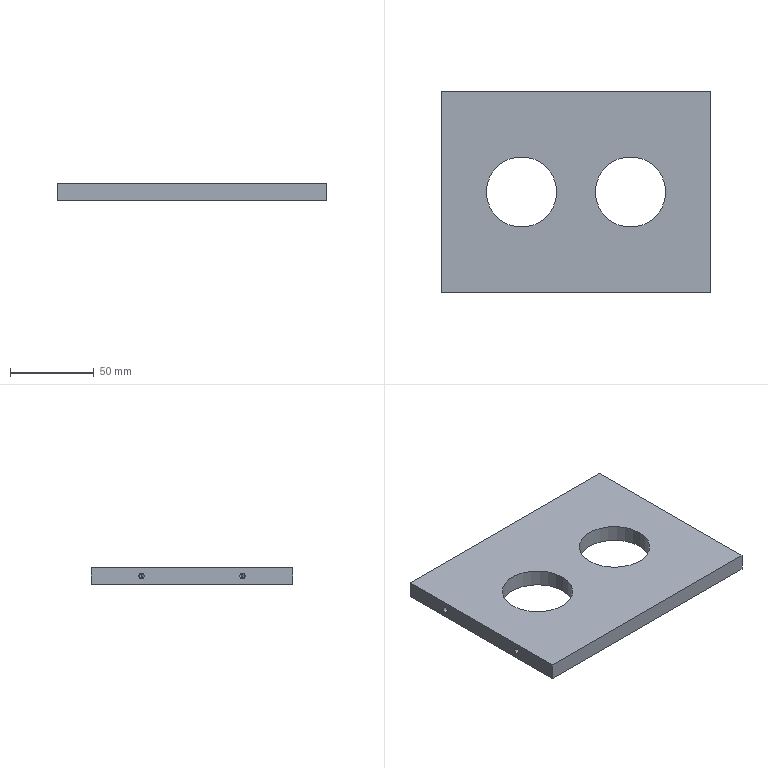Part | NX | 1 solid | 26 faces | box 160 x 120 x 10 mm | volume 163934 mm3 | cylinder 12 | cone 8 | plane 6 | commonest cylinder face diameters 3.3 x8 42 x4
STEP:
#1=CARTESIAN_POINT('',(-69.9,-30.,3.35));
#2=VERTEX_POINT('',#1);
#3=CARTESIAN_POINT('',(-69.9,-30.,6.65));
#4=VERTEX_POINT('',#3);
#5=CARTESIAN_POINT('',(-69.9,-30.,5.));
#6=DIRECTION('',(-1.,0.,0.));
#7=DIRECTION('',(0.,0.,1.));
#8=AXIS2_PLACEMENT_3D('',#5,#6,#7);
#9=CIRCLE('',#8,1.65);
#10=EDGE_CURVE('',#2,#4,#9,.T.);
#11=ORIENTED_EDGE('',*,*,#10,.F.);
#12=CARTESIAN_POINT('',(-80.,-30.,3.35));
#13=VERTEX_POINT('',#12);
#14=CARTESIAN_POINT('',(-80.,-30.,3.35));
#15=DIRECTION('',(-1.,0.,0.));
#16=VECTOR('',#15,1.);
#17=LINE('',#14,#16);
#18=EDGE_CURVE('',#2,#13,#17,.T.);
#19=ORIENTED_EDGE('',*,*,#18,.T.);
#20=CARTESIAN_POINT('',(-80.,-30.,6.65));
#21=VERTEX_POINT('',#20);
#22=CARTESIAN_POINT('',(-80.,-30.,5.));
#23=DIRECTION('',(-1.,0.,0.));
#24=DIRECTION('',(0.,0.,1.));
#25=AXIS2_PLACEMENT_3D('',#22,#23,#24);
#26=CIRCLE('',#25,1.65);
#27=EDGE_CURVE('',#13,#21,#26,.T.);
#28=ORIENTED_EDGE('',*,*,#27,.T.);
#29=CARTESIAN_POINT('',(-80.,-30.,6.65));
#30=DIRECTION('',(-1.,0.,0.));
#31=VECTOR('',#30,1.);
#32=LINE('',#29,#31);
#33=EDGE_CURVE('',#4,#21,#32,.T.);
#34=ORIENTED_EDGE('',*,*,#33,.F.);
#35=EDGE_LOOP('',(#11,#19,#28,#34));
#36=FACE_OUTER_BOUND('',#35,.T.);
#37=CARTESIAN_POINT('',(-80.,-30.,5.));
#38=DIRECTION('',(-1.,0.,0.));
#39=DIRECTION('',(0.,0.,1.));
#40=AXIS2_PLACEMENT_3D('',#37,#38,#39);
#41=CYLINDRICAL_SURFACE('',#40,1.65);
#42=ADVANCED_FACE('',(#36),#41,.F.);
#43=CARTESIAN_POINT('',(-68.909,-30.,5.));
#44=VERTEX_POINT('',#43);
#45=CARTESIAN_POINT('',(-69.9,-30.,6.65));
#46=DIRECTION('',(-0.515,0.,0.8572));
#47=VECTOR('',#46,1.);
#48=LINE('',#45,#47);
#49=EDGE_CURVE('',#44,#4,#48,.T.);
#50=ORIENTED_EDGE('',*,*,#49,.F.);
#51=CARTESIAN_POINT('',(-69.9,-30.,3.35));
#52=DIRECTION('',(-0.515,0.,-0.8572));
#53=VECTOR('',#52,1.);
#54=LINE('',#51,#53);
#55=EDGE_CURVE('',#44,#2,#54,.T.);
#56=ORIENTED_EDGE('',*,*,#55,.T.);
#57=ORIENTED_EDGE('',*,*,#10,.T.);
#58=EDGE_LOOP('',(#50,#56,#57));
#59=FACE_OUTER_BOUND('',#58,.T.);
#60=CARTESIAN_POINT('',(-69.9,-30.,5.));
#61=DIRECTION('',(-1.,0.,0.));
#62=DIRECTION('',(0.,0.,1.));
#63=AXIS2_PLACEMENT_3D('',#60,#61,#62);
#64=CONICAL_SURFACE('',#63,1.65,59.);
#65=ADVANCED_FACE('',(#59),#64,.F.);
#66=CARTESIAN_POINT('',(-69.9,30.,3.35));
#67=VERTEX_POINT('',#66);
#68=CARTESIAN_POINT('',(-69.9,30.,6.65));
#69=VERTEX_POINT('',#68);
#70=CARTESIAN_POINT('',(-69.9,30.,5.));
#71=DIRECTION('',(-1.,0.,0.));
#72=DIRECTION('',(0.,0.,1.));
#73=AXIS2_PLACEMENT_3D('',#70,#71,#72);
#74=CIRCLE('',#73,1.65);
#75=EDGE_CURVE('',#67,#69,#74,.T.);
#76=ORIENTED_EDGE('',*,*,#75,.F.);
#77=CARTESIAN_POINT('',(-80.,30.,3.35));
#78=VERTEX_POINT('',#77);
#79=CARTESIAN_POINT('',(-80.,30.,3.35));
#80=DIRECTION('',(-1.,0.,0.));
#81=VECTOR('',#80,1.);
#82=LINE('',#79,#81);
#83=EDGE_CURVE('',#67,#78,#82,.T.);
#84=ORIENTED_EDGE('',*,*,#83,.T.);
#85=CARTESIAN_POINT('',(-80.,30.,6.65));
#86=VERTEX_POINT('',#85);
#87=CARTESIAN_POINT('',(-80.,30.,5.));
#88=DIRECTION('',(-1.,0.,0.));
#89=DIRECTION('',(0.,0.,1.));
#90=AXIS2_PLACEMENT_3D('',#87,#88,#89);
#91=CIRCLE('',#90,1.65);
#92=EDGE_CURVE('',#78,#86,#91,.T.);
#93=ORIENTED_EDGE('',*,*,#92,.T.);
#94=CARTESIAN_POINT('',(-80.,30.,6.65));
#95=DIRECTION('',(-1.,0.,0.));
#96=VECTOR('',#95,1.);
#97=LINE('',#94,#96);
#98=EDGE_CURVE('',#69,#86,#97,.T.);
#99=ORIENTED_EDGE('',*,*,#98,.F.);
#100=EDGE_LOOP('',(#76,#84,#93,#99));
#101=FACE_OUTER_BOUND('',#100,.T.);
#102=CARTESIAN_POINT('',(-80.,30.,5.));
#103=DIRECTION('',(-1.,0.,0.));
#104=DIRECTION('',(0.,0.,1.));
#105=AXIS2_PLACEMENT_3D('',#102,#103,#104);
#106=CYLINDRICAL_SURFACE('',#105,1.65);
#107=ADVANCED_FACE('',(#101),#106,.F.);
#108=CARTESIAN_POINT('',(-68.909,30.,5.));
#109=VERTEX_POINT('',#108);
#110=CARTESIAN_POINT('',(-69.9,30.,6.65));
#111=DIRECTION('',(-0.515,0.,0.8572));
#112=VECTOR('',#111,1.);
#113=LINE('',#110,#112);
#114=EDGE_CURVE('',#109,#69,#113,.T.);
#115=ORIENTED_EDGE('',*,*,#114,.F.);
#116=CARTESIAN_POINT('',(-69.9,30.,3.35));
#117=DIRECTION('',(-0.515,0.,-0.8572));
#118=VECTOR('',#117,1.);
#119=LINE('',#116,#118);
#120=EDGE_CURVE('',#109,#67,#119,.T.);
#121=ORIENTED_EDGE('',*,*,#120,.T.);
#122=ORIENTED_EDGE('',*,*,#75,.T.);
#123=EDGE_LOOP('',(#115,#121,#122));
#124=FACE_OUTER_BOUND('',#123,.T.);
#125=CARTESIAN_POINT('',(-69.9,30.,5.));
#126=DIRECTION('',(-1.,0.,0.));
#127=DIRECTION('',(0.,0.,1.));
#128=AXIS2_PLACEMENT_3D('',#125,#126,#127);
#129=CONICAL_SURFACE('',#128,1.65,59.);
#130=ADVANCED_FACE('',(#124),#129,.F.);
#131=CARTESIAN_POINT('',(69.9,-30.,6.65));
#132=VERTEX_POINT('',#131);
#133=CARTESIAN_POINT('',(69.9,-30.,3.35));
#134=VERTEX_POINT('',#133);
#135=CARTESIAN_POINT('',(69.9,-30.,5.));
#136=DIRECTION('',(1.,0.,0.));
#137=DIRECTION('',(0.,0.,-1.));
#138=AXIS2_PLACEMENT_3D('',#135,#136,#137);
#139=CIRCLE('',#138,1.65);
#140=EDGE_CURVE('',#132,#134,#139,.T.);
#141=ORIENTED_EDGE('',*,*,#140,.F.);
#142=CARTESIAN_POINT('',(80.,-30.,6.65));
#143=VERTEX_POINT('',#142);
#144=CARTESIAN_POINT('',(80.,-30.,6.65));
#145=DIRECTION('',(-1.,0.,0.));
#146=VECTOR('',#145,1.);
#147=LINE('',#144,#146);
#148=EDGE_CURVE('',#143,#132,#147,.T.);
#149=ORIENTED_EDGE('',*,*,#148,.F.);
#150=CARTESIAN_POINT('',(80.,-30.,3.35));
#151=VERTEX_POINT('',#150);
#152=CARTESIAN_POINT('',(80.,-30.,5.));
#153=DIRECTION('',(1.,0.,0.));
#154=DIRECTION('',(0.,0.,-1.));
#155=AXIS2_PLACEMENT_3D('',#152,#153,#154);
#156=CIRCLE('',#155,1.65);
#157=EDGE_CURVE('',#143,#151,#156,.T.);
#158=ORIENTED_EDGE('',*,*,#157,.T.);
#159=CARTESIAN_POINT('',(80.,-30.,3.35));
#160=DIRECTION('',(-1.,0.,0.));
#161=VECTOR('',#160,1.);
#162=LINE('',#159,#161);
#163=EDGE_CURVE('',#151,#134,#162,.T.);
#164=ORIENTED_EDGE('',*,*,#163,.T.);
#165=EDGE_LOOP('',(#141,#149,#158,#164));
#166=FACE_OUTER_BOUND('',#165,.T.);
#167=CARTESIAN_POINT('',(80.,-30.,5.));
#168=DIRECTION('',(1.,0.,0.));
#169=DIRECTION('',(0.,0.,-1.));
#170=AXIS2_PLACEMENT_3D('',#167,#168,#169);
#171=CYLINDRICAL_SURFACE('',#170,1.65);
#172=ADVANCED_FACE('',(#166),#171,.F.);
#173=CARTESIAN_POINT('',(68.909,-30.,5.));
#174=VERTEX_POINT('',#173);
#175=CARTESIAN_POINT('',(69.9,-30.,3.35));
#176=DIRECTION('',(-0.515,0.,0.8572));
#177=VECTOR('',#176,1.);
#178=LINE('',#175,#177);
#179=EDGE_CURVE('',#134,#174,#178,.T.);
#180=ORIENTED_EDGE('',*,*,#179,.T.);
#181=CARTESIAN_POINT('',(69.9,-30.,6.65));
#182=DIRECTION('',(-0.515,0.,-0.8572));
#183=VECTOR('',#182,1.);
#184=LINE('',#181,#183);
#185=EDGE_CURVE('',#132,#174,#184,.T.);
#186=ORIENTED_EDGE('',*,*,#185,.F.);
#187=ORIENTED_EDGE('',*,*,#140,.T.);
#188=EDGE_LOOP('',(#180,#186,#187));
#189=FACE_OUTER_BOUND('',#188,.T.);
#190=CARTESIAN_POINT('',(69.9,-30.,5.));
#191=DIRECTION('',(1.,0.,0.));
#192=DIRECTION('',(0.,0.,-1.));
#193=AXIS2_PLACEMENT_3D('',#190,#191,#192);
#194=CONICAL_SURFACE('',#193,1.65,59.);
#195=ADVANCED_FACE('',(#189),#194,.F.);
#196=CARTESIAN_POINT('',(69.9,30.,6.65));
#197=VERTEX_POINT('',#196);
#198=CARTESIAN_POINT('',(69.9,30.,3.35));
#199=VERTEX_POINT('',#198);
#200=CARTESIAN_POINT('',(69.9,30.,5.));
#201=DIRECTION('',(1.,0.,0.));
#202=DIRECTION('',(0.,0.,-1.));
#203=AXIS2_PLACEMENT_3D('',#200,#201,#202);
#204=CIRCLE('',#203,1.65);
#205=EDGE_CURVE('',#197,#199,#204,.T.);
#206=ORIENTED_EDGE('',*,*,#205,.F.);
#207=CARTESIAN_POINT('',(80.,30.,6.65));
#208=VERTEX_POINT('',#207);
#209=CARTESIAN_POINT('',(80.,30.,6.65));
#210=DIRECTION('',(-1.,0.,0.));
#211=VECTOR('',#210,1.);
#212=LINE('',#209,#211);
#213=EDGE_CURVE('',#208,#197,#212,.T.);
#214=ORIENTED_EDGE('',*,*,#213,.F.);
#215=CARTESIAN_POINT('',(80.,30.,3.35));
#216=VERTEX_POINT('',#215);
#217=CARTESIAN_POINT('',(80.,30.,5.));
#218=DIRECTION('',(1.,0.,0.));
#219=DIRECTION('',(0.,0.,-1.));
#220=AXIS2_PLACEMENT_3D('',#217,#218,#219);
#221=CIRCLE('',#220,1.65);
#222=EDGE_CURVE('',#208,#216,#221,.T.);
#223=ORIENTED_EDGE('',*,*,#222,.T.);
#224=CARTESIAN_POINT('',(80.,30.,3.35));
#225=DIRECTION('',(-1.,0.,0.));
#226=VECTOR('',#225,1.);
#227=LINE('',#224,#226);
#228=EDGE_CURVE('',#216,#199,#227,.T.);
#229=ORIENTED_EDGE('',*,*,#228,.T.);
#230=EDGE_LOOP('',(#206,#214,#223,#229));
#231=FACE_OUTER_BOUND('',#230,.T.);
#232=CARTESIAN_POINT('',(80.,30.,5.));
#233=DIRECTION('',(1.,0.,0.));
#234=DIRECTION('',(0.,0.,-1.));
#235=AXIS2_PLACEMENT_3D('',#232,#233,#234);
#236=CYLINDRICAL_SURFACE('',#235,1.65);
#237=ADVANCED_FACE('',(#231),#236,.F.);
#238=CARTESIAN_POINT('',(68.909,30.,5.));
#239=VERTEX_POINT('',#238);
#240=CARTESIAN_POINT('',(69.9,30.,3.35));
#241=DIRECTION('',(-0.515,0.,0.8572));
#242=VECTOR('',#241,1.);
#243=LINE('',#240,#242);
#244=EDGE_CURVE('',#199,#239,#243,.T.);
#245=ORIENTED_EDGE('',*,*,#244,.T.);
#246=CARTESIAN_POINT('',(69.9,30.,6.65));
#247=DIRECTION('',(-0.515,0.,-0.8572));
#248=VECTOR('',#247,1.);
#249=LINE('',#246,#248);
#250=EDGE_CURVE('',#197,#239,#249,.T.);
#251=ORIENTED_EDGE('',*,*,#250,.F.);
#252=ORIENTED_EDGE('',*,*,#205,.T.);
#253=EDGE_LOOP('',(#245,#251,#252));
#254=FACE_OUTER_BOUND('',#253,.T.);
#255=CARTESIAN_POINT('',(69.9,30.,5.));
#256=DIRECTION('',(1.,0.,0.));
#257=DIRECTION('',(0.,0.,-1.));
#258=AXIS2_PLACEMENT_3D('',#255,#256,#257);
#259=CONICAL_SURFACE('',#258,1.65,59.);
#260=ADVANCED_FACE('',(#254),#259,.F.);
#261=CARTESIAN_POINT('',(-53.5,0.,10.));
#262=VERTEX_POINT('',#261);
#263=CARTESIAN_POINT('',(-11.5,0.,10.));
#264=VERTEX_POINT('',#263);
#265=CARTESIAN_POINT('',(-32.5,0.,10.));
#266=DIRECTION('',(0.,0.,1.));
#267=DIRECTION('',(1.,0.,0.));
#268=AXIS2_PLACEMENT_3D('',#265,#266,#267);
#269=CIRCLE('',#268,21.);
#270=EDGE_CURVE('',#262,#264,#269,.T.);
#271=ORIENTED_EDGE('',*,*,#270,.T.);
#272=CARTESIAN_POINT('',(-11.5,0.,0.));
#273=VERTEX_POINT('',#272);
#274=CARTESIAN_POINT('',(-11.5,0.,10.));
#275=DIRECTION('',(0.,0.,1.));
#276=VECTOR('',#275,1.);
#277=LINE('',#274,#276);
#278=EDGE_CURVE('',#273,#264,#277,.T.);
#279=ORIENTED_EDGE('',*,*,#278,.F.);
#280=CARTESIAN_POINT('',(-53.5,0.,0.));
#281=VERTEX_POINT('',#280);
#282=CARTESIAN_POINT('',(-32.5,0.,0.));
#283=DIRECTION('',(0.,0.,1.));
#284=DIRECTION('',(1.,0.,0.));
#285=AXIS2_PLACEMENT_3D('',#282,#283,#284);
#286=CIRCLE('',#285,21.);
#287=EDGE_CURVE('',#281,#273,#286,.T.);
#288=ORIENTED_EDGE('',*,*,#287,.F.);
#289=CARTESIAN_POINT('',(-53.5,0.,10.));
#290=DIRECTION('',(0.,0.,1.));
#291=VECTOR('',#290,1.);
#292=LINE('',#289,#291);
#293=EDGE_CURVE('',#281,#262,#292,.T.);
#294=ORIENTED_EDGE('',*,*,#293,.T.);
#295=EDGE_LOOP('',(#271,#279,#288,#294));
#296=FACE_OUTER_BOUND('',#295,.T.);
#297=CARTESIAN_POINT('',(-32.5,0.,10.));
#298=DIRECTION('',(0.,0.,-1.));
#299=DIRECTION('',(-1.,0.,0.));
#300=AXIS2_PLACEMENT_3D('',#297,#298,#299);
#301=CYLINDRICAL_SURFACE('',#300,21.);
#302=ADVANCED_FACE('',(#296),#301,.F.);
#303=CARTESIAN_POINT('',(11.5,0.,10.));
#304=VERTEX_POINT('',#303);
#305=CARTESIAN_POINT('',(53.5,0.,10.));
#306=VERTEX_POINT('',#305);
#307=CARTESIAN_POINT('',(32.5,0.,10.));
#308=DIRECTION('',(0.,0.,1.));
#309=DIRECTION('',(1.,0.,0.));
#310=AXIS2_PLACEMENT_3D('',#307,#308,#309);
#311=CIRCLE('',#310,21.);
#312=EDGE_CURVE('',#304,#306,#311,.T.);
#313=ORIENTED_EDGE('',*,*,#312,.T.);
#314=CARTESIAN_POINT('',(53.5,0.,0.));
#315=VERTEX_POINT('',#314);
#316=CARTESIAN_POINT('',(53.5,0.,10.));
#317=DIRECTION('',(0.,0.,1.));
#318=VECTOR('',#317,1.);
#319=LINE('',#316,#318);
#320=EDGE_CURVE('',#315,#306,#319,.T.);
#321=ORIENTED_EDGE('',*,*,#320,.F.);
#322=CARTESIAN_POINT('',(11.5,0.,0.));
#323=VERTEX_POINT('',#322);
#324=CARTESIAN_POINT('',(32.5,0.,0.));
#325=DIRECTION('',(0.,0.,1.));
#326=DIRECTION('',(1.,0.,0.));
#327=AXIS2_PLACEMENT_3D('',#324,#325,#326);
#328=CIRCLE('',#327,21.);
#329=EDGE_CURVE('',#323,#315,#328,.T.);
#330=ORIENTED_EDGE('',*,*,#329,.F.);
#331=CARTESIAN_POINT('',(11.5,0.,10.));
#332=DIRECTION('',(0.,0.,1.));
#333=VECTOR('',#332,1.);
#334=LINE('',#331,#333);
#335=EDGE_CURVE('',#323,#304,#334,.T.);
#336=ORIENTED_EDGE('',*,*,#335,.T.);
#337=EDGE_LOOP('',(#313,#321,#330,#336));
#338=FACE_OUTER_BOUND('',#337,.T.);
#339=CARTESIAN_POINT('',(32.5,0.,10.));
#340=DIRECTION('',(0.,0.,-1.));
#341=DIRECTION('',(-1.,0.,0.));
#342=AXIS2_PLACEMENT_3D('',#339,#340,#341);
#343=CYLINDRICAL_SURFACE('',#342,21.);
#344=ADVANCED_FACE('',(#338),#343,.F.);
#345=ORIENTED_EDGE('',*,*,#312,.F.);
#346=CARTESIAN_POINT('',(32.5,0.,10.));
#347=DIRECTION('',(0.,0.,1.));
#348=DIRECTION('',(1.,0.,0.));
#349=AXIS2_PLACEMENT_3D('',#346,#347,#348);
#350=CIRCLE('',#349,21.);
#351=EDGE_CURVE('',#306,#304,#350,.T.);
#352=ORIENTED_EDGE('',*,*,#351,.F.);
#353=EDGE_LOOP('',(#345,#352));
#354=FACE_BOUND('',#353,.T.);
#355=CARTESIAN_POINT('',(80.,-60.,10.));
#356=VERTEX_POINT('',#355);
#357=CARTESIAN_POINT('',(80.,60.,10.));
#358=VERTEX_POINT('',#357);
#359=CARTESIAN_POINT('',(80.,60.,10.));
#360=DIRECTION('',(0.,1.,0.));
#361=VECTOR('',#360,1.);
#362=LINE('',#359,#361);
#363=EDGE_CURVE('',#356,#358,#362,.T.);
#364=ORIENTED_EDGE('',*,*,#363,.T.);
#365=CARTESIAN_POINT('',(-80.,60.,10.));
#366=VERTEX_POINT('',#365);
#367=CARTESIAN_POINT('',(-80.,60.,10.));
#368=DIRECTION('',(-1.,0.,0.));
#369=VECTOR('',#368,1.);
#370=LINE('',#367,#369);
#371=EDGE_CURVE('',#358,#366,#370,.T.);
#372=ORIENTED_EDGE('',*,*,#371,.T.);
#373=CARTESIAN_POINT('',(-80.,-60.,10.));
#374=VERTEX_POINT('',#373);
#375=CARTESIAN_POINT('',(-80.,60.,10.));
#376=DIRECTION('',(0.,-1.,0.));
#377=VECTOR('',#376,1.);
#378=LINE('',#375,#377);
#379=EDGE_CURVE('',#366,#374,#378,.T.);
#380=ORIENTED_EDGE('',*,*,#379,.T.);
#381=CARTESIAN_POINT('',(-80.,-60.,10.));
#382=DIRECTION('',(1.,0.,0.));
#383=VECTOR('',#382,1.);
#384=LINE('',#381,#383);
#385=EDGE_CURVE('',#374,#356,#384,.T.);
#386=ORIENTED_EDGE('',*,*,#385,.T.);
#387=EDGE_LOOP('',(#364,#372,#380,#386));
#388=FACE_BOUND('',#387,.T.);
#389=ORIENTED_EDGE('',*,*,#270,.F.);
#390=CARTESIAN_POINT('',(-32.5,0.,10.));
#391=DIRECTION('',(0.,0.,1.));
#392=DIRECTION('',(1.,0.,0.));
#393=AXIS2_PLACEMENT_3D('',#390,#391,#392);
#394=CIRCLE('',#393,21.);
#395=EDGE_CURVE('',#264,#262,#394,.T.);
#396=ORIENTED_EDGE('',*,*,#395,.F.);
#397=EDGE_LOOP('',(#389,#396));
#398=FACE_BOUND('',#397,.T.);
#399=CARTESIAN_POINT('',(80.,-60.,10.));
#400=DIRECTION('',(0.,0.,1.));
#401=DIRECTION('',(1.,0.,0.));
#402=AXIS2_PLACEMENT_3D('',#399,#400,#401);
#403=PLANE('',#402);
#404=ADVANCED_FACE('',(#354,#388,#398),#403,.T.);
#405=ORIENTED_EDGE('',*,*,#329,.T.);
#406=CARTESIAN_POINT('',(32.5,0.,0.));
#407=DIRECTION('',(0.,0.,1.));
#408=DIRECTION('',(1.,0.,0.));
#409=AXIS2_PLACEMENT_3D('',#406,#407,#408);
#410=CIRCLE('',#409,21.);
#411=EDGE_CURVE('',#315,#323,#410,.T.);
#412=ORIENTED_EDGE('',*,*,#411,.T.);
#413=EDGE_LOOP('',(#405,#412));
#414=FACE_BOUND('',#413,.T.);
#415=CARTESIAN_POINT('',(80.,-60.,0.));
#416=VERTEX_POINT('',#415);
#417=CARTESIAN_POINT('',(80.,60.,0.));
#418=VERTEX_POINT('',#417);
#419=CARTESIAN_POINT('',(80.,60.,0.));
#420=DIRECTION('',(0.,1.,0.));
#421=VECTOR('',#420,1.);
#422=LINE('',#419,#421);
#423=EDGE_CURVE('',#416,#418,#422,.T.);
#424=ORIENTED_EDGE('',*,*,#423,.F.);
#425=CARTESIAN_POINT('',(-80.,-60.,0.));
#426=VERTEX_POINT('',#425);
#427=CARTESIAN_POINT('',(-80.,-60.,0.));
#428=DIRECTION('',(1.,0.,0.));
#429=VECTOR('',#428,1.);
#430=LINE('',#427,#429);
#431=EDGE_CURVE('',#426,#416,#430,.T.);
#432=ORIENTED_EDGE('',*,*,#431,.F.);
#433=CARTESIAN_POINT('',(-80.,60.,0.));
#434=VERTEX_POINT('',#433);
#435=CARTESIAN_POINT('',(-80.,60.,0.));
#436=DIRECTION('',(0.,-1.,0.));
#437=VECTOR('',#436,1.);
#438=LINE('',#435,#437);
#439=EDGE_CURVE('',#434,#426,#438,.T.);
#440=ORIENTED_EDGE('',*,*,#439,.F.);
#441=CARTESIAN_POINT('',(-80.,60.,0.));
#442=DIRECTION('',(-1.,0.,0.));
#443=VECTOR('',#442,1.);
#444=LINE('',#441,#443);
#445=EDGE_CURVE('',#418,#434,#444,.T.);
#446=ORIENTED_EDGE('',*,*,#445,.F.);
#447=EDGE_LOOP('',(#424,#432,#440,#446));
#448=FACE_BOUND('',#447,.T.);
#449=ORIENTED_EDGE('',*,*,#287,.T.);
#450=CARTESIAN_POINT('',(-32.5,0.,0.));
#451=DIRECTION('',(0.,0.,1.));
#452=DIRECTION('',(1.,0.,0.));
#453=AXIS2_PLACEMENT_3D('',#450,#451,#452);
#454=CIRCLE('',#453,21.);
#455=EDGE_CURVE('',#273,#281,#454,.T.);
#456=ORIENTED_EDGE('',*,*,#455,.T.);
#457=EDGE_LOOP('',(#449,#456));
#458=FACE_BOUND('',#457,.T.);
#459=CARTESIAN_POINT('',(80.,-60.,0.));
#460=DIRECTION('',(0.,0.,1.));
#461=DIRECTION('',(1.,0.,0.));
#462=AXIS2_PLACEMENT_3D('',#459,#460,#461);
#463=PLANE('',#462);
#464=ADVANCED_FACE('',(#414,#448,#458),#463,.F.);
#465=CARTESIAN_POINT('',(80.,-30.,5.));
#466=DIRECTION('',(1.,0.,0.));
#467=DIRECTION('',(0.,0.,-1.));
#468=AXIS2_PLACEMENT_3D('',#465,#466,#467);
#469=CIRCLE('',#468,1.65);
#470=EDGE_CURVE('',#151,#143,#469,.T.);
#471=ORIENTED_EDGE('',*,*,#470,.F.);
#472=ORIENTED_EDGE('',*,*,#157,.F.);
#473=EDGE_LOOP('',(#471,#472));
#474=FACE_BOUND('',#473,.T.);
#475=CARTESIAN_POINT('',(80.,30.,5.));
#476=DIRECTION('',(1.,0.,0.));
#477=DIRECTION('',(0.,0.,-1.));
#478=AXIS2_PLACEMENT_3D('',#475,#476,#477);
#479=CIRCLE('',#478,1.65);
#480=EDGE_CURVE('',#216,#208,#479,.T.);
#481=ORIENTED_EDGE('',*,*,#480,.F.);
#482=ORIENTED_EDGE('',*,*,#222,.F.);
#483=EDGE_LOOP('',(#481,#482));
#484=FACE_BOUND('',#483,.T.);
#485=ORIENTED_EDGE('',*,*,#423,.T.);
#486=CARTESIAN_POINT('',(80.,60.,10.));
#487=DIRECTION('',(0.,0.,-1.));
#488=VECTOR('',#487,1.);
#489=LINE('',#486,#488);
#490=EDGE_CURVE('',#358,#418,#489,.T.);
#491=ORIENTED_EDGE('',*,*,#490,.F.);
#492=ORIENTED_EDGE('',*,*,#363,.F.);
#493=CARTESIAN_POINT('',(80.,-60.,10.));
#494=DIRECTION('',(0.,0.,-1.));
#495=VECTOR('',#494,1.);
#496=LINE('',#493,#495);
#497=EDGE_CURVE('',#356,#416,#496,.T.);
#498=ORIENTED_EDGE('',*,*,#497,.T.);
#499=EDGE_LOOP('',(#485,#491,#492,#498));
#500=FACE_BOUND('',#499,.T.);
#501=CARTESIAN_POINT('',(80.,60.,10.));
#502=DIRECTION('',(-1.,0.,0.));
#503=DIRECTION('',(0.,-1.,0.));
#504=AXIS2_PLACEMENT_3D('',#501,#502,#503);
#505=PLANE('',#504);
#506=ADVANCED_FACE('',(#474,#484,#500),#505,.F.);
#507=ORIENTED_EDGE('',*,*,#445,.T.);
#508=CARTESIAN_POINT('',(-80.,60.,10.));
#509=DIRECTION('',(0.,0.,-1.));
#510=VECTOR('',#509,1.);
#511=LINE('',#508,#510);
#512=EDGE_CURVE('',#366,#434,#511,.T.);
#513=ORIENTED_EDGE('',*,*,#512,.F.);
#514=ORIENTED_EDGE('',*,*,#371,.F.);
#515=ORIENTED_EDGE('',*,*,#490,.T.);
#516=EDGE_LOOP('',(#507,#513,#514,#515));
#517=FACE_OUTER_BOUND('',#516,.T.);
#518=CARTESIAN_POINT('',(-80.,60.,10.));
#519=DIRECTION('',(0.,-1.,0.));
#520=DIRECTION('',(1.,0.,0.));
#521=AXIS2_PLACEMENT_3D('',#518,#519,#520);
#522=PLANE('',#521);
#523=ADVANCED_FACE('',(#517),#522,.F.);
#524=CARTESIAN_POINT('',(-80.,-30.,5.));
#525=DIRECTION('',(-1.,0.,0.));
#526=DIRECTION('',(0.,0.,1.));
#527=AXIS2_PLACEMENT_3D('',#524,#525,#526);
#528=CIRCLE('',#527,1.65);
#529=EDGE_CURVE('',#21,#13,#528,.T.);
#530=ORIENTED_EDGE('',*,*,#529,.F.);
#531=ORIENTED_EDGE('',*,*,#27,.F.);
#532=EDGE_LOOP('',(#530,#531));
#533=FACE_BOUND('',#532,.T.);
#534=CARTESIAN_POINT('',(-80.,30.,5.));
#535=DIRECTION('',(-1.,0.,0.));
#536=DIRECTION('',(0.,0.,1.));
#537=AXIS2_PLACEMENT_3D('',#534,#535,#536);
#538=CIRCLE('',#537,1.65);
#539=EDGE_CURVE('',#86,#78,#538,.T.);
#540=ORIENTED_EDGE('',*,*,#539,.F.);
#541=ORIENTED_EDGE('',*,*,#92,.F.);
#542=EDGE_LOOP('',(#540,#541));
#543=FACE_BOUND('',#542,.T.);
#544=ORIENTED_EDGE('',*,*,#439,.T.);
#545=CARTESIAN_POINT('',(-80.,-60.,10.));
#546=DIRECTION('',(0.,0.,-1.));
#547=VECTOR('',#546,1.);
#548=LINE('',#545,#547);
#549=EDGE_CURVE('',#374,#426,#548,.T.);
#550=ORIENTED_EDGE('',*,*,#549,.F.);
#551=ORIENTED_EDGE('',*,*,#379,.F.);
#552=ORIENTED_EDGE('',*,*,#512,.T.);
#553=EDGE_LOOP('',(#544,#550,#551,#552));
#554=FACE_BOUND('',#553,.T.);
#555=CARTESIAN_POINT('',(-80.,60.,10.));
#556=DIRECTION('',(1.,0.,0.));
#557=DIRECTION('',(0.,1.,0.));
#558=AXIS2_PLACEMENT_3D('',#555,#556,#557);
#559=PLANE('',#558);
#560=ADVANCED_FACE('',(#533,#543,#554),#559,.F.);
#561=ORIENTED_EDGE('',*,*,#431,.T.);
#562=ORIENTED_EDGE('',*,*,#497,.F.);
#563=ORIENTED_EDGE('',*,*,#385,.F.);
#564=ORIENTED_EDGE('',*,*,#549,.T.);
#565=EDGE_LOOP('',(#561,#562,#563,#564));
#566=FACE_OUTER_BOUND('',#565,.T.);
#567=CARTESIAN_POINT('',(-80.,-60.,10.));
#568=DIRECTION('',(0.,1.,0.));
#569=DIRECTION('',(-1.,0.,0.));
#570=AXIS2_PLACEMENT_3D('',#567,#568,#569);
#571=PLANE('',#570);
#572=ADVANCED_FACE('',(#566),#571,.F.);
#573=ORIENTED_EDGE('',*,*,#320,.T.);
#574=ORIENTED_EDGE('',*,*,#351,.T.);
#575=ORIENTED_EDGE('',*,*,#335,.F.);
#576=ORIENTED_EDGE('',*,*,#411,.F.);
#577=EDGE_LOOP('',(#573,#574,#575,#576));
#578=FACE_OUTER_BOUND('',#577,.T.);
#579=CARTESIAN_POINT('',(32.5,0.,10.));
#580=DIRECTION('',(0.,0.,-1.));
#581=DIRECTION('',(-1.,0.,0.));
#582=AXIS2_PLACEMENT_3D('',#579,#580,#581);
#583=CYLINDRICAL_SURFACE('',#582,21.);
#584=ADVANCED_FACE('',(#578),#583,.F.);
#585=ORIENTED_EDGE('',*,*,#278,.T.);
#586=ORIENTED_EDGE('',*,*,#395,.T.);
#587=ORIENTED_EDGE('',*,*,#293,.F.);
#588=ORIENTED_EDGE('',*,*,#455,.F.);
#589=EDGE_LOOP('',(#585,#586,#587,#588));
#590=FACE_OUTER_BOUND('',#589,.T.);
#591=CARTESIAN_POINT('',(-32.5,0.,10.));
#592=DIRECTION('',(0.,0.,-1.));
#593=DIRECTION('',(-1.,0.,0.));
#594=AXIS2_PLACEMENT_3D('',#591,#592,#593);
#595=CYLINDRICAL_SURFACE('',#594,21.);
#596=ADVANCED_FACE('',(#590),#595,.F.);
#597=ORIENTED_EDGE('',*,*,#250,.T.);
#598=ORIENTED_EDGE('',*,*,#244,.F.);
#599=CARTESIAN_POINT('',(69.9,30.,5.));
#600=DIRECTION('',(1.,0.,0.));
#601=DIRECTION('',(0.,0.,-1.));
#602=AXIS2_PLACEMENT_3D('',#599,#600,#601);
#603=CIRCLE('',#602,1.65);
#604=EDGE_CURVE('',#199,#197,#603,.T.);
#605=ORIENTED_EDGE('',*,*,#604,.T.);
#606=EDGE_LOOP('',(#597,#598,#605));
#607=FACE_OUTER_BOUND('',#606,.T.);
#608=CARTESIAN_POINT('',(69.9,30.,5.));
#609=DIRECTION('',(1.,0.,0.));
#610=DIRECTION('',(0.,0.,-1.));
#611=AXIS2_PLACEMENT_3D('',#608,#609,#610);
#612=CONICAL_SURFACE('',#611,1.65,59.);
#613=ADVANCED_FACE('',(#607),#612,.F.);
#614=ORIENTED_EDGE('',*,*,#213,.T.);
#615=ORIENTED_EDGE('',*,*,#604,.F.);
#616=ORIENTED_EDGE('',*,*,#228,.F.);
#617=ORIENTED_EDGE('',*,*,#480,.T.);
#618=EDGE_LOOP('',(#614,#615,#616,#617));
#619=FACE_OUTER_BOUND('',#618,.T.);
#620=CARTESIAN_POINT('',(80.,30.,5.));
#621=DIRECTION('',(1.,0.,0.));
#622=DIRECTION('',(0.,0.,-1.));
#623=AXIS2_PLACEMENT_3D('',#620,#621,#622);
#624=CYLINDRICAL_SURFACE('',#623,1.65);
#625=ADVANCED_FACE('',(#619),#624,.F.);
#626=ORIENTED_EDGE('',*,*,#185,.T.);
#627=ORIENTED_EDGE('',*,*,#179,.F.);
#628=CARTESIAN_POINT('',(69.9,-30.,5.));
#629=DIRECTION('',(1.,0.,0.));
#630=DIRECTION('',(0.,0.,-1.));
#631=AXIS2_PLACEMENT_3D('',#628,#629,#630);
#632=CIRCLE('',#631,1.65);
#633=EDGE_CURVE('',#134,#132,#632,.T.);
#634=ORIENTED_EDGE('',*,*,#633,.T.);
#635=EDGE_LOOP('',(#626,#627,#634));
#636=FACE_OUTER_BOUND('',#635,.T.);
#637=CARTESIAN_POINT('',(69.9,-30.,5.));
#638=DIRECTION('',(1.,0.,0.));
#639=DIRECTION('',(0.,0.,-1.));
#640=AXIS2_PLACEMENT_3D('',#637,#638,#639);
#641=CONICAL_SURFACE('',#640,1.65,59.);
#642=ADVANCED_FACE('',(#636),#641,.F.);
#643=ORIENTED_EDGE('',*,*,#148,.T.);
#644=ORIENTED_EDGE('',*,*,#633,.F.);
#645=ORIENTED_EDGE('',*,*,#163,.F.);
#646=ORIENTED_EDGE('',*,*,#470,.T.);
#647=EDGE_LOOP('',(#643,#644,#645,#646));
#648=FACE_OUTER_BOUND('',#647,.T.);
#649=CARTESIAN_POINT('',(80.,-30.,5.));
#650=DIRECTION('',(1.,0.,0.));
#651=DIRECTION('',(0.,0.,-1.));
#652=AXIS2_PLACEMENT_3D('',#649,#650,#651);
#653=CYLINDRICAL_SURFACE('',#652,1.65);
#654=ADVANCED_FACE('',(#648),#653,.F.);
#655=ORIENTED_EDGE('',*,*,#120,.F.);
#656=ORIENTED_EDGE('',*,*,#114,.T.);
#657=CARTESIAN_POINT('',(-69.9,30.,5.));
#658=DIRECTION('',(-1.,0.,0.));
#659=DIRECTION('',(0.,0.,1.));
#660=AXIS2_PLACEMENT_3D('',#657,#658,#659);
#661=CIRCLE('',#660,1.65);
#662=EDGE_CURVE('',#69,#67,#661,.T.);
#663=ORIENTED_EDGE('',*,*,#662,.T.);
#664=EDGE_LOOP('',(#655,#656,#663));
#665=FACE_OUTER_BOUND('',#664,.T.);
#666=CARTESIAN_POINT('',(-69.9,30.,5.));
#667=DIRECTION('',(-1.,0.,0.));
#668=DIRECTION('',(0.,0.,1.));
#669=AXIS2_PLACEMENT_3D('',#666,#667,#668);
#670=CONICAL_SURFACE('',#669,1.65,59.);
#671=ADVANCED_FACE('',(#665),#670,.F.);
#672=ORIENTED_EDGE('',*,*,#83,.F.);
#673=ORIENTED_EDGE('',*,*,#662,.F.);
#674=ORIENTED_EDGE('',*,*,#98,.T.);
#675=ORIENTED_EDGE('',*,*,#539,.T.);
#676=EDGE_LOOP('',(#672,#673,#674,#675));
#677=FACE_OUTER_BOUND('',#676,.T.);
#678=CARTESIAN_POINT('',(-80.,30.,5.));
#679=DIRECTION('',(-1.,0.,0.));
#680=DIRECTION('',(0.,0.,1.));
#681=AXIS2_PLACEMENT_3D('',#678,#679,#680);
#682=CYLINDRICAL_SURFACE('',#681,1.65);
#683=ADVANCED_FACE('',(#677),#682,.F.);
#684=ORIENTED_EDGE('',*,*,#18,.F.);
#685=CARTESIAN_POINT('',(-69.9,-30.,5.));
#686=DIRECTION('',(-1.,0.,0.));
#687=DIRECTION('',(0.,0.,1.));
#688=AXIS2_PLACEMENT_3D('',#685,#686,#687);
#689=CIRCLE('',#688,1.65);
#690=EDGE_CURVE('',#4,#2,#689,.T.);
#691=ORIENTED_EDGE('',*,*,#690,.F.);
#692=ORIENTED_EDGE('',*,*,#33,.T.);
#693=ORIENTED_EDGE('',*,*,#529,.T.);
#694=EDGE_LOOP('',(#684,#691,#692,#693));
#695=FACE_OUTER_BOUND('',#694,.T.);
#696=CARTESIAN_POINT('',(-80.,-30.,5.));
#697=DIRECTION('',(-1.,0.,0.));
#698=DIRECTION('',(0.,0.,1.));
#699=AXIS2_PLACEMENT_3D('',#696,#697,#698);
#700=CYLINDRICAL_SURFACE('',#699,1.65);
#701=ADVANCED_FACE('',(#695),#700,.F.);
#702=ORIENTED_EDGE('',*,*,#55,.F.);
#703=ORIENTED_EDGE('',*,*,#49,.T.);
#704=ORIENTED_EDGE('',*,*,#690,.T.);
#705=EDGE_LOOP('',(#702,#703,#704));
#706=FACE_OUTER_BOUND('',#705,.T.);
#707=CARTESIAN_POINT('',(-69.9,-30.,5.));
#708=DIRECTION('',(-1.,0.,0.));
#709=DIRECTION('',(0.,0.,1.));
#710=AXIS2_PLACEMENT_3D('',#707,#708,#709);
#711=CONICAL_SURFACE('',#710,1.65,59.);
#712=ADVANCED_FACE('',(#706),#711,.F.);
#713=CLOSED_SHELL('',(#42,#65,#107,#130,#172,#195,#237,#260,#302,#344,#404,#464,#506,#523,#560,#572,#584,#596,#613,#625,#642,#654,#671,#683,#701,#712));
#714=MANIFOLD_SOLID_BREP('',#713);
#715=(LENGTH_UNIT()NAMED_UNIT(*)SI_UNIT(.MILLI.,.METRE.));
#716=UNCERTAINTY_MEASURE_WITH_UNIT(LENGTH_MEASURE(0.00002),#715,'','');
#717=(NAMED_UNIT(*)PLANE_ANGLE_UNIT()SI_UNIT($,.RADIAN.));
#718=PLANE_ANGLE_MEASURE_WITH_UNIT(PLANE_ANGLE_MEASURE(0.01745),#717);
#719=DIMENSIONAL_EXPONENTS(0.,0.,0.,0.,0.,0.,0.);
#720=(CONVERSION_BASED_UNIT('DEGREE',#718)NAMED_UNIT(#719)PLANE_ANGLE_UNIT());
#721=(NAMED_UNIT(*)SI_UNIT($,.STERADIAN.)SOLID_ANGLE_UNIT());
#722=(GEOMETRIC_REPRESENTATION_CONTEXT(3)GLOBAL_UNCERTAINTY_ASSIGNED_CONTEXT((#716))GLOBAL_UNIT_ASSIGNED_CONTEXT((#715,#720,#721))REPRESENTATION_CONTEXT('',''));
#723=ADVANCED_BREP_SHAPE_REPRESENTATION('',(#714),#722);